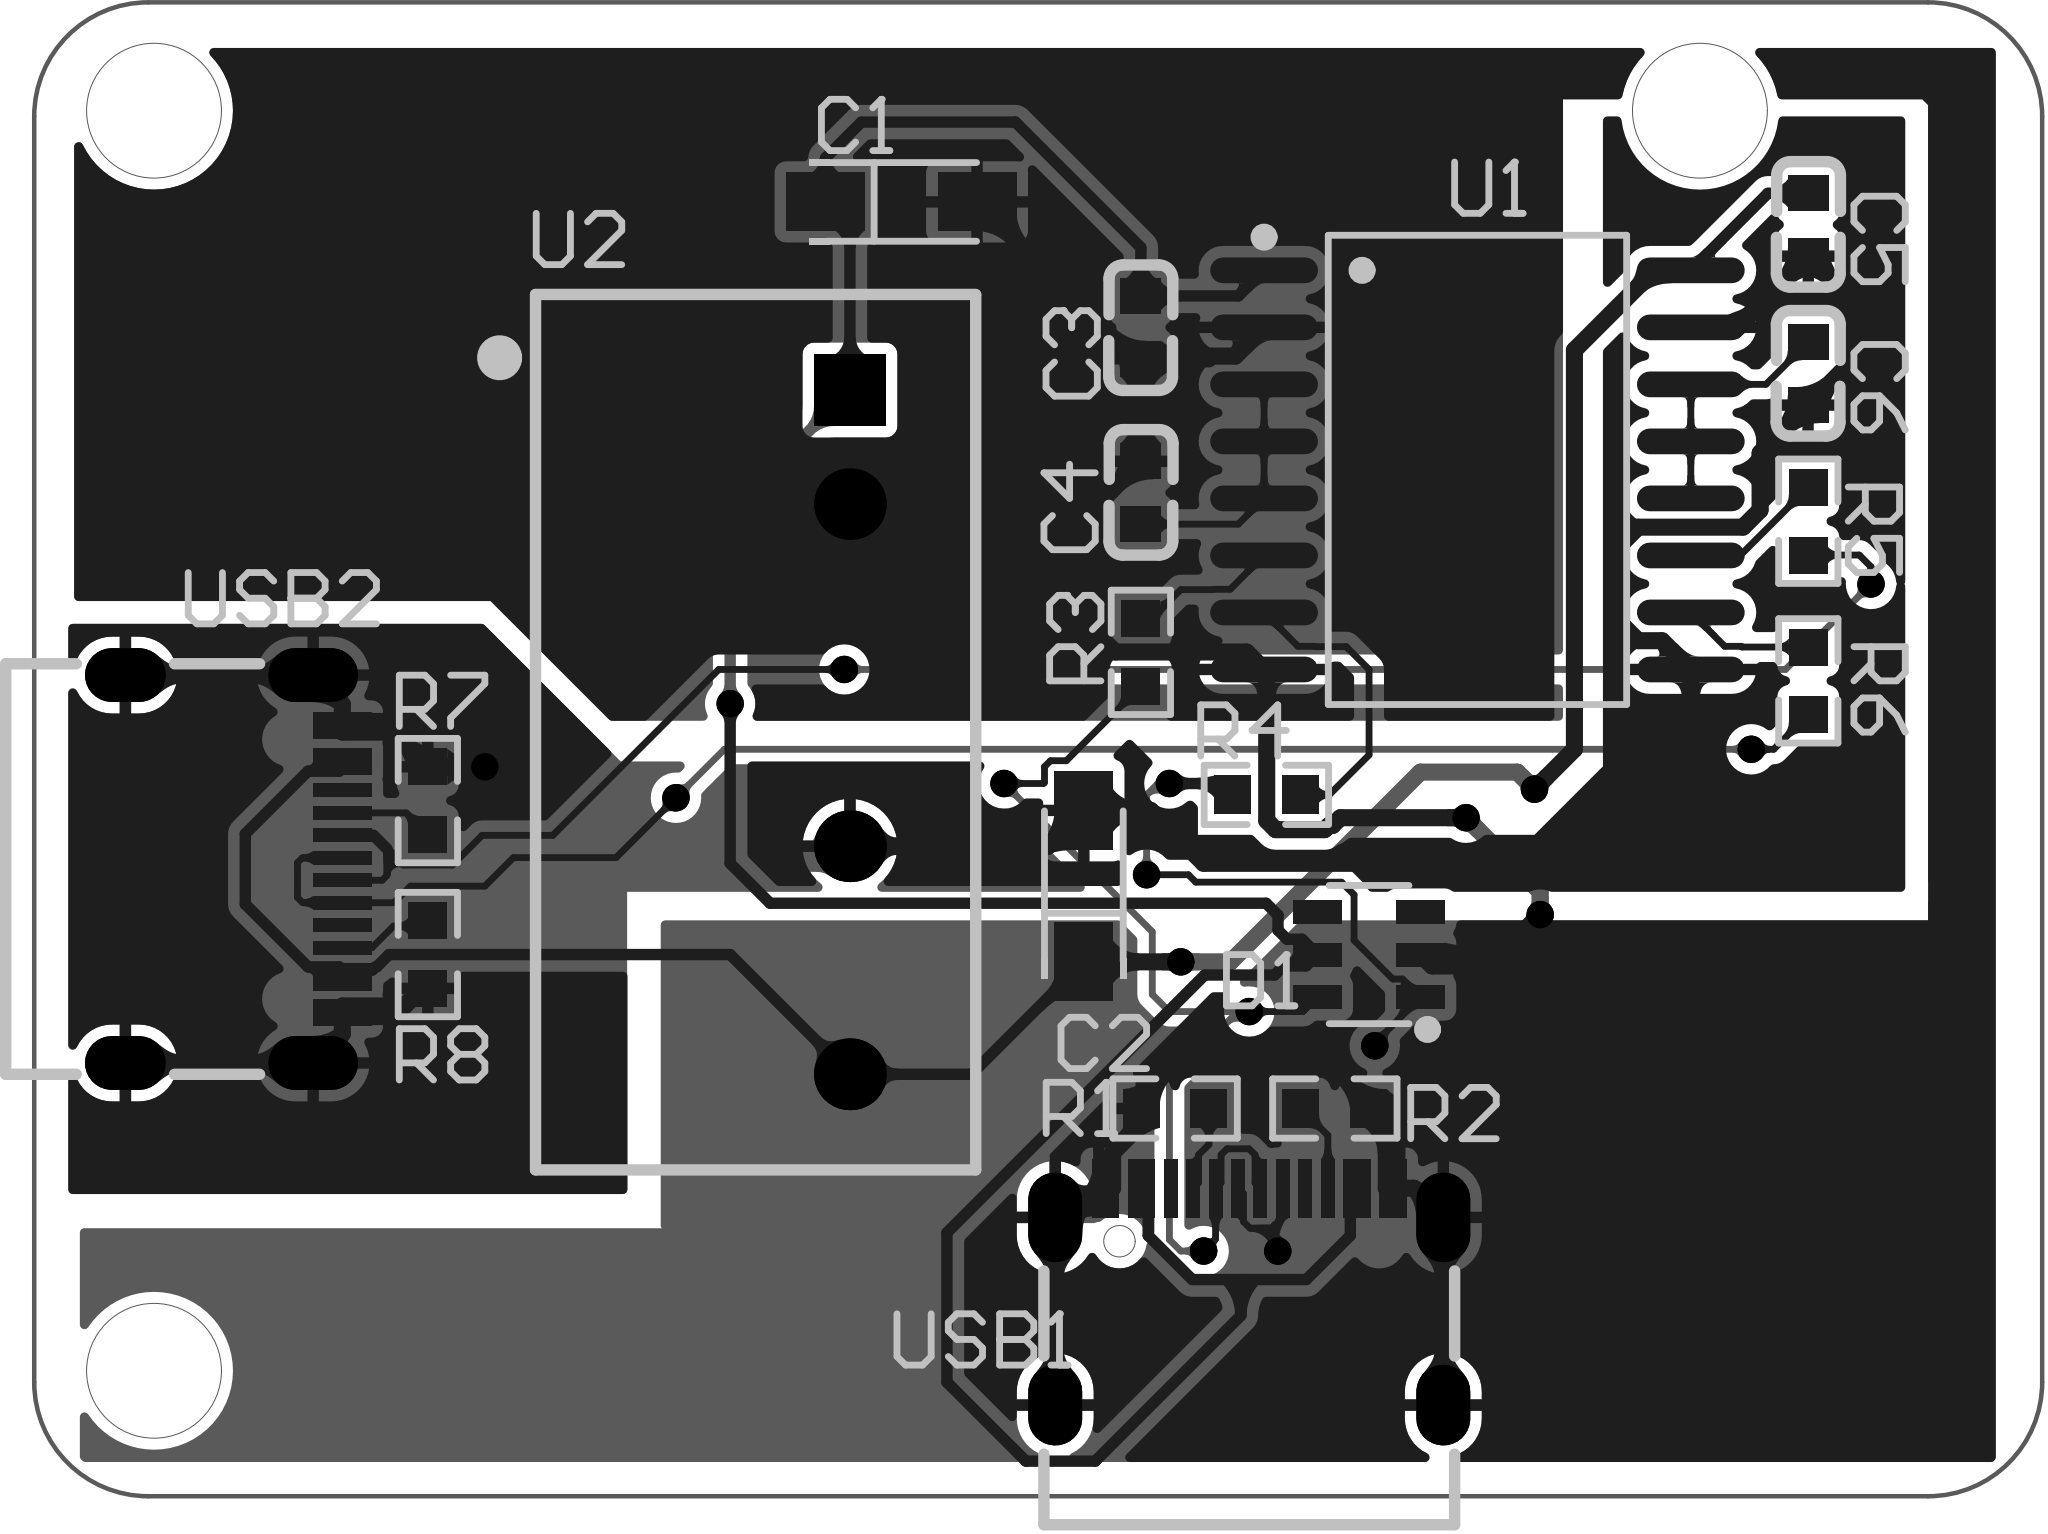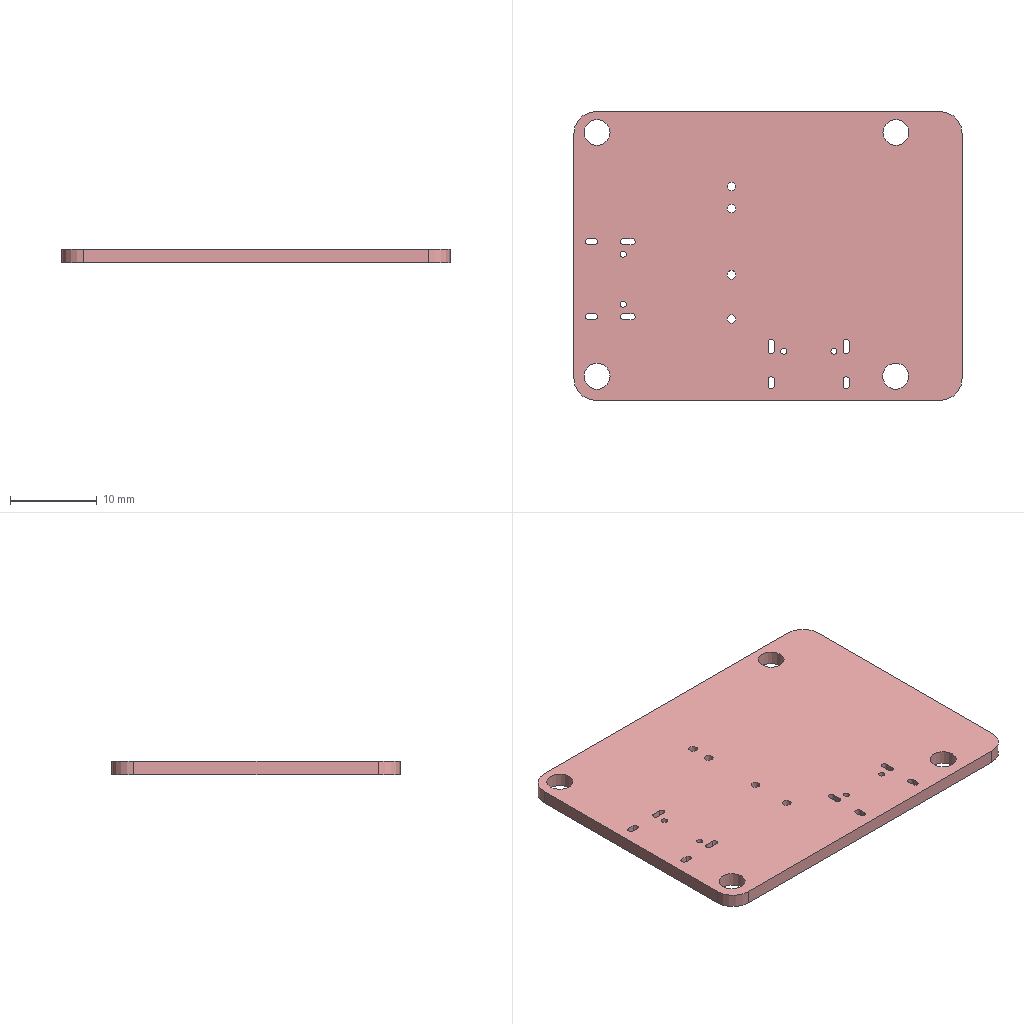Circuit board layout | Altium Designer | box 44.7 x 33.3 x 1.6 mm
Layer stack:
# Altium Designer layer stack of  (unit mm; dielectric type: 0 none, 1 core, 2 prepreg, 3 surface material)
index,name,kind,layer,copper_thickness_mm,dielectric_type,dielectric_thickness_mm,dielectric_material,dielectric_constant
0,Top Paste Mask Layer,other,,,,,,
1,Top Silkscreen Layer,other,,,,,,
2,Top Solder Mask Layer,dielectric,,,3,0.01,,3.3
3,Top Layer,copper,Top Layer,0.035,,,,
4,Dielectric1,dielectric,,,3,1.51,FR4,4.5
5,Bottom Layer,copper,Bottom Layer,0.035,,,,
6,Bottom Solder Mask Layer,dielectric,,,3,0.01,,3.3
7,Bottom Silkscreen Layer,other,,,,,,
8,Bottom Paste Mask Layer,other,,,,,,
# drill layer pairs: low layer,high layer
drill_pair,Top Layer,Bottom Layer
Part placement:
Designator,Comment,Layer,Footprint,Center-X(mm),Center-Y(mm),Rotation
C1,10uF,TopLayer,CAP-SMD_L3.2-W1.6-RD-C7171,96.139,105.664,0
C2,10uF,TopLayer,CAP-SMD_L3.2-W1.6-RD-C7171,100.203,90.424,90
C3,100nF,TopLayer,C0603,101.473,102.87,90
C4,100nF,TopLayer,C0603,101.473,99.187,270
C5,100nF,TopLayer,C0603,116.332,105.156,270
C6,100nF,TopLayer,C0603,116.327,101.839,270
D1,SRV05-4HTG,TopLayer,SOT-23-6_L2.9-W1.6-P0.95-LS2.8-BL,106.553,88.9,90
R3,24Ω,TopLayer,R0603,101.473,95.631,90
R4,24Ω,TopLayer,R0603,104.267,92.456,0
R5,24Ω,TopLayer,R0603,116.332,98.552,270
R6,24Ω,TopLayer,R0603,116.332,94.996,270
U1,ADUM4160BRWZ-RL,TopLayer,SOIC-16_L10.3-W7.5-P1.27-LS10.3-BL,108.966,99.695,270
U2,H0505S-2WR2,TopLayer,PWRM-TH_EVISUN_HXXXXS-2WR2,94.996,93.853,270
USB1,KH-TYPE-C-16P,TopLayer,USB-C-SMD_KH-TYPE-C-16P,103.886,81.28,0
USB2,KH-TYPE-C-16P,TopLayer,USB-C-SMD_KH-TYPE-C-16P,81.28,90.805,270
R1,10K,TopLayer,R0603,102.235,85.471,180
R2,10K,TopLayer,R0603,105.791,85.471,180
R7,10K,TopLayer,R0603,85.598,92.329,90
R8,10K,TopLayer,R0603,85.598,88.9,90
Pad and via stacks:
# Altium Designer via and pad stacks of  (unit mm). Each distinct definition once, with the count of objects using it.
# via: kind,start_layer,end_layer,hole_mm,diameter_mm,mode(0 simple;1 top-mid-bottom;2 full stack),diameter_per_layer,count,example_net
# pad: kind,layer,hole_mm,hole_type(0 round;1 square;2 slot),plating,top_size,top_shape(1 round;2 rect;3 octagon;9 rounded rect),mid_size,bottom_size,mode,footprint,size_per_layer,count,example
pad,Top Layer,0,0,plated,1.758x1.296,2,1.758x1.296,1.758x1.296,0,CAP-SMD_L3.2-W1.6-RD-C7171,,4,C1.1
pad,Top Layer,0,0,plated,0.8x0.9,2,0.8x0.9,0.8x0.9,0,C0603,,8,C3.2
pad,Top Layer,0,0,plated,0.532x1.072,2,0.532x1.072,0.532x1.072,0,SOT-23-6_L2.9-W1.6-P0.95-LS2.8-BL,,6,D1.1
pad,Top Layer,0,0,plated,0.8065x0.864,2,0.8065x0.864,0.8065x0.864,0,R0603,,16,R3.2
pad,Top Layer,0,0,plated,0.574x2.401,1,0.574x2.401,0.574x2.401,0,SOIC-16_L10.3-W7.5-P1.27-LS10.3-BL,,16,U1.1
pad,Top Layer,0,0,plated,0.3x1.3,2,0.3x1.3,0.3x1.3,0,USB-C-SMD_KH-TYPE-C-16P,,32,USB1.A1
pad,Multi-Layer,1,0,plated,1.6x1.6,1,1.6x1.6,1.6x1.6,0,PWRM-TH_EVISUN_HXXXXS-2WR2,,3,U2.7
pad,Multi-Layer,1,0,plated,1.6x1.6,2,1.6x1.6,1.6x1.6,0,PWRM-TH_EVISUN_HXXXXS-2WR2,,1,U2.1
pad,Multi-Layer,0.7,2,plated,1.2x1.8,1,1.2x1.8,1.2x1.8,0,USB-C-SMD_KH-TYPE-C-16P,,4,USB1.3
pad,Multi-Layer,0.7,2,plated,1.2x2,1,1.2x2,1.2x2,0,USB-C-SMD_KH-TYPE-C-16P,,4,USB1.2
via,Top Layer,Bottom Layer,0.3048,0.61,0,,17,+5V-USB
Copper pours:
name,layer,net,type(0 solid;1 hatched;2 none)
Top Layer-GND,Top Layer,GND,0
Top Layer-GND-USB,Top Layer,GND-USB,0
Bottom Layer-GND,Bottom Layer,GND,0
Bottom Layer-GND-USB,Bottom Layer,GND-USB,0